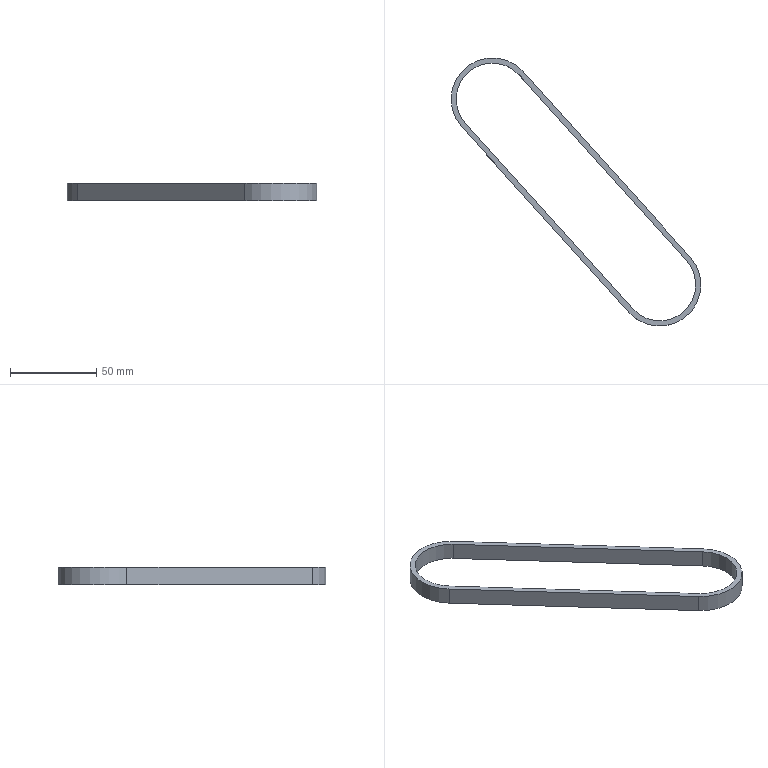Part | STEP file | 1 solid | 12 faces | box 145.075 x 155.71 x 10 mm | volume 12941 mm3 | plane 6 | cylinder 6 | commonest cylinder face diameters 42 x3 48 x3
STEP:
#1=CARTESIAN_POINT('',(0.,0.,0.));
#2=DIRECTION('',(0.,0.,1.));
#3=DIRECTION('',(1.,0.,0.));
#4=AXIS2_PLACEMENT_3D('',#1,#2,#3);
#5=CARTESIAN_POINT('',(15.599,14.059,-2.));
#6=VERTEX_POINT('',#5);
#7=CARTESIAN_POINT('',(-81.476,121.769,-2.));
#8=VERTEX_POINT('',#7);
#9=CARTESIAN_POINT('',(15.599,14.059,-2.));
#10=DIRECTION('',(-0.6695,0.7428,0.));
#11=VECTOR('',#10,1.);
#12=LINE('',#9,#11);
#13=CARTESIAN_POINT('',(15.599,14.059,-12.));
#14=DIRECTION('',(0.7428,0.6695,0.));
#15=DIRECTION('',(0.,0.,-1.));
#16=AXIS2_PLACEMENT_3D('',#13,#14,#15);
#17=PLANE('',#16);
#18=CARTESIAN_POINT('',(-10.,0.));
#19=DIRECTION('',(0.,1.));
#20=VECTOR('',#19,1.);
#21=LINE('',#18,#20);
#22=(GEOMETRIC_REPRESENTATION_CONTEXT(2)PARAMETRIC_REPRESENTATION_CONTEXT()REPRESENTATION_CONTEXT('',''));
#23=DEFINITIONAL_REPRESENTATION('',(#21),#22);
#24=PCURVE('',#17,#23);
#25=CARTESIAN_POINT('',(0.,0.,-2.));
#26=DIRECTION('',(0.,0.,1.));
#27=DIRECTION('',(1.,0.,0.));
#28=AXIS2_PLACEMENT_3D('',#25,#26,#27);
#29=PLANE('',#28);
#30=CARTESIAN_POINT('',(15.599,14.059));
#31=DIRECTION('',(-0.6695,0.7428));
#32=VECTOR('',#31,1.);
#33=LINE('',#30,#32);
#34=(GEOMETRIC_REPRESENTATION_CONTEXT(2)PARAMETRIC_REPRESENTATION_CONTEXT()REPRESENTATION_CONTEXT('',''));
#35=DEFINITIONAL_REPRESENTATION('',(#33),#34);
#36=PCURVE('',#29,#35);
#37=SURFACE_CURVE('',#12,(#24,#36),.PCURVE_S1.);
#38=EDGE_CURVE('',#6,#8,#37,.T.);
#39=ORIENTED_EDGE('',*,*,#38,.T.);
#40=CARTESIAN_POINT('',(-81.476,121.769,-12.));
#41=VERTEX_POINT('',#40);
#42=CARTESIAN_POINT('',(-81.476,121.769,-12.));
#43=DIRECTION('',(0.,0.,1.));
#44=VECTOR('',#43,1.);
#45=LINE('',#42,#44);
#46=CARTESIAN_POINT('',(0.,145.));
#47=DIRECTION('',(-1.,0.));
#48=VECTOR('',#47,1.);
#49=LINE('',#46,#48);
#50=(GEOMETRIC_REPRESENTATION_CONTEXT(2)PARAMETRIC_REPRESENTATION_CONTEXT()REPRESENTATION_CONTEXT('',''));
#51=DEFINITIONAL_REPRESENTATION('',(#49),#50);
#52=PCURVE('',#17,#51);
#53=CARTESIAN_POINT('',(-97.075,107.71,-12.));
#54=DIRECTION('',(0.,0.,1.));
#55=DIRECTION('',(1.,0.,0.));
#56=AXIS2_PLACEMENT_3D('',#53,#54,#55);
#57=CYLINDRICAL_SURFACE('',#56,21.);
#58=CARTESIAN_POINT('',(0.7335,0.));
#59=DIRECTION('',(0.,1.));
#60=VECTOR('',#59,1.);
#61=LINE('',#58,#60);
#62=(GEOMETRIC_REPRESENTATION_CONTEXT(2)PARAMETRIC_REPRESENTATION_CONTEXT()REPRESENTATION_CONTEXT('',''));
#63=DEFINITIONAL_REPRESENTATION('',(#61),#62);
#64=PCURVE('',#57,#63);
#65=SURFACE_CURVE('',#45,(#52,#64),.PCURVE_S1.);
#66=EDGE_CURVE('',#41,#8,#65,.T.);
#67=ORIENTED_EDGE('',*,*,#66,.F.);
#68=CARTESIAN_POINT('',(15.599,14.059,-12.));
#69=VERTEX_POINT('',#68);
#70=CARTESIAN_POINT('',(15.599,14.059,-12.));
#71=DIRECTION('',(-0.6695,0.7428,0.));
#72=VECTOR('',#71,1.);
#73=LINE('',#70,#72);
#74=CARTESIAN_POINT('',(0.,0.));
#75=DIRECTION('',(0.,1.));
#76=VECTOR('',#75,1.);
#77=LINE('',#74,#76);
#78=(GEOMETRIC_REPRESENTATION_CONTEXT(2)PARAMETRIC_REPRESENTATION_CONTEXT()REPRESENTATION_CONTEXT('',''));
#79=DEFINITIONAL_REPRESENTATION('',(#77),#78);
#80=PCURVE('',#17,#79);
#81=CARTESIAN_POINT('',(0.,0.,-12.));
#82=DIRECTION('',(0.,0.,1.));
#83=DIRECTION('',(1.,0.,0.));
#84=AXIS2_PLACEMENT_3D('',#81,#82,#83);
#85=PLANE('',#84);
#86=CARTESIAN_POINT('',(15.599,14.059));
#87=DIRECTION('',(-0.6695,0.7428));
#88=VECTOR('',#87,1.);
#89=LINE('',#86,#88);
#90=(GEOMETRIC_REPRESENTATION_CONTEXT(2)PARAMETRIC_REPRESENTATION_CONTEXT()REPRESENTATION_CONTEXT('',''));
#91=DEFINITIONAL_REPRESENTATION('',(#89),#90);
#92=PCURVE('',#85,#91);
#93=SURFACE_CURVE('',#73,(#80,#92),.PCURVE_S1.);
#94=EDGE_CURVE('',#69,#41,#93,.T.);
#95=ORIENTED_EDGE('',*,*,#94,.F.);
#96=CARTESIAN_POINT('',(15.599,14.059,-12.));
#97=DIRECTION('',(0.,0.,1.));
#98=VECTOR('',#97,1.);
#99=LINE('',#96,#98);
#100=CARTESIAN_POINT('',(0.,0.));
#101=DIRECTION('',(-1.,0.));
#102=VECTOR('',#101,1.);
#103=LINE('',#100,#102);
#104=(GEOMETRIC_REPRESENTATION_CONTEXT(2)PARAMETRIC_REPRESENTATION_CONTEXT()REPRESENTATION_CONTEXT('',''));
#105=DEFINITIONAL_REPRESENTATION('',(#103),#104);
#106=PCURVE('',#17,#105);
#107=CARTESIAN_POINT('',(0.,0.,-12.));
#108=DIRECTION('',(0.,0.,1.));
#109=DIRECTION('',(1.,0.,0.));
#110=AXIS2_PLACEMENT_3D('',#107,#108,#109);
#111=CYLINDRICAL_SURFACE('',#110,21.);
#112=CARTESIAN_POINT('',(0.7335,0.));
#113=DIRECTION('',(0.,1.));
#114=VECTOR('',#113,1.);
#115=LINE('',#112,#114);
#116=(GEOMETRIC_REPRESENTATION_CONTEXT(2)PARAMETRIC_REPRESENTATION_CONTEXT()REPRESENTATION_CONTEXT('',''));
#117=DEFINITIONAL_REPRESENTATION('',(#115),#116);
#118=PCURVE('',#111,#117);
#119=SURFACE_CURVE('',#99,(#106,#118),.PCURVE_S1.);
#120=EDGE_CURVE('',#69,#6,#119,.T.);
#121=ORIENTED_EDGE('',*,*,#120,.T.);
#122=EDGE_LOOP('',(#39,#67,#95,#121));
#123=FACE_BOUND('',#122,.T.);
#124=ADVANCED_FACE('',(#123),#17,.F.);
#125=ORIENTED_EDGE('',*,*,#66,.F.);
#126=CARTESIAN_POINT('',(-112.674,93.651,-12.));
#127=VERTEX_POINT('',#126);
#128=CARTESIAN_POINT('',(-97.075,107.71,-12.));
#129=DIRECTION('',(0.,0.,1.));
#130=DIRECTION('',(1.,0.,0.));
#131=AXIS2_PLACEMENT_3D('',#128,#129,#130);
#132=CIRCLE('',#131,21.);
#133=CARTESIAN_POINT('',(0.,0.));
#134=DIRECTION('',(1.,0.));
#135=VECTOR('',#134,1.);
#136=LINE('',#133,#135);
#137=(GEOMETRIC_REPRESENTATION_CONTEXT(2)PARAMETRIC_REPRESENTATION_CONTEXT()REPRESENTATION_CONTEXT('',''));
#138=DEFINITIONAL_REPRESENTATION('',(#136),#137);
#139=PCURVE('',#57,#138);
#140=CARTESIAN_POINT('',(-97.075,107.71));
#141=DIRECTION('',(1.,0.));
#142=AXIS2_PLACEMENT_2D('',#140,#141);
#143=CIRCLE('',#142,21.);
#144=(GEOMETRIC_REPRESENTATION_CONTEXT(2)PARAMETRIC_REPRESENTATION_CONTEXT()REPRESENTATION_CONTEXT('',''));
#145=DEFINITIONAL_REPRESENTATION('',(#143),#144);
#146=PCURVE('',#85,#145);
#147=SURFACE_CURVE('',#132,(#139,#146),.PCURVE_S1.);
#148=EDGE_CURVE('',#41,#127,#147,.T.);
#149=ORIENTED_EDGE('',*,*,#148,.T.);
#150=CARTESIAN_POINT('',(-112.674,93.651,-2.));
#151=VERTEX_POINT('',#150);
#152=CARTESIAN_POINT('',(-112.674,93.651,-12.));
#153=DIRECTION('',(0.,0.,1.));
#154=VECTOR('',#153,1.);
#155=LINE('',#152,#154);
#156=CARTESIAN_POINT('',(3.875,0.));
#157=DIRECTION('',(0.,1.));
#158=VECTOR('',#157,1.);
#159=LINE('',#156,#158);
#160=(GEOMETRIC_REPRESENTATION_CONTEXT(2)PARAMETRIC_REPRESENTATION_CONTEXT()REPRESENTATION_CONTEXT('',''));
#161=DEFINITIONAL_REPRESENTATION('',(#159),#160);
#162=PCURVE('',#57,#161);
#163=CARTESIAN_POINT('',(-15.599,-14.059,-12.));
#164=DIRECTION('',(-0.7428,-0.6695,0.));
#165=DIRECTION('',(-0.6695,0.7428,0.));
#166=AXIS2_PLACEMENT_3D('',#163,#164,#165);
#167=PLANE('',#166);
#168=CARTESIAN_POINT('',(145.,0.));
#169=DIRECTION('',(0.,-1.));
#170=VECTOR('',#169,1.);
#171=LINE('',#168,#170);
#172=(GEOMETRIC_REPRESENTATION_CONTEXT(2)PARAMETRIC_REPRESENTATION_CONTEXT()REPRESENTATION_CONTEXT('',''));
#173=DEFINITIONAL_REPRESENTATION('',(#171),#172);
#174=PCURVE('',#167,#173);
#175=SURFACE_CURVE('',#155,(#162,#174),.PCURVE_S1.);
#176=EDGE_CURVE('',#127,#151,#175,.T.);
#177=ORIENTED_EDGE('',*,*,#176,.T.);
#178=CARTESIAN_POINT('',(-97.075,107.71,-2.));
#179=DIRECTION('',(0.,0.,1.));
#180=DIRECTION('',(1.,0.,0.));
#181=AXIS2_PLACEMENT_3D('',#178,#179,#180);
#182=CIRCLE('',#181,21.);
#183=CARTESIAN_POINT('',(0.,10.));
#184=DIRECTION('',(1.,0.));
#185=VECTOR('',#184,1.);
#186=LINE('',#183,#185);
#187=(GEOMETRIC_REPRESENTATION_CONTEXT(2)PARAMETRIC_REPRESENTATION_CONTEXT()REPRESENTATION_CONTEXT('',''));
#188=DEFINITIONAL_REPRESENTATION('',(#186),#187);
#189=PCURVE('',#57,#188);
#190=CARTESIAN_POINT('',(-97.075,107.71));
#191=DIRECTION('',(1.,0.));
#192=AXIS2_PLACEMENT_2D('',#190,#191);
#193=CIRCLE('',#192,21.);
#194=(GEOMETRIC_REPRESENTATION_CONTEXT(2)PARAMETRIC_REPRESENTATION_CONTEXT()REPRESENTATION_CONTEXT('',''));
#195=DEFINITIONAL_REPRESENTATION('',(#193),#194);
#196=PCURVE('',#29,#195);
#197=SURFACE_CURVE('',#182,(#189,#196),.PCURVE_S1.);
#198=EDGE_CURVE('',#8,#151,#197,.T.);
#199=ORIENTED_EDGE('',*,*,#198,.F.);
#200=EDGE_LOOP('',(#125,#149,#177,#199));
#201=FACE_BOUND('',#200,.F.);
#202=ADVANCED_FACE('',(#201),#57,.F.);
#203=CARTESIAN_POINT('',(-15.599,-14.059,-2.));
#204=VERTEX_POINT('',#203);
#205=CARTESIAN_POINT('',(-15.599,-14.059,-2.));
#206=DIRECTION('',(0.6695,-0.7428,0.));
#207=VECTOR('',#206,1.);
#208=LINE('',#205,#207);
#209=CARTESIAN_POINT('',(0.,-10.));
#210=DIRECTION('',(-1.,0.));
#211=VECTOR('',#210,1.);
#212=LINE('',#209,#211);
#213=(GEOMETRIC_REPRESENTATION_CONTEXT(2)PARAMETRIC_REPRESENTATION_CONTEXT()REPRESENTATION_CONTEXT('',''));
#214=DEFINITIONAL_REPRESENTATION('',(#212),#213);
#215=PCURVE('',#167,#214);
#216=CARTESIAN_POINT('',(-15.599,-14.059));
#217=DIRECTION('',(0.6695,-0.7428));
#218=VECTOR('',#217,1.);
#219=LINE('',#216,#218);
#220=(GEOMETRIC_REPRESENTATION_CONTEXT(2)PARAMETRIC_REPRESENTATION_CONTEXT()REPRESENTATION_CONTEXT('',''));
#221=DEFINITIONAL_REPRESENTATION('',(#219),#220);
#222=PCURVE('',#29,#221);
#223=SURFACE_CURVE('',#208,(#215,#222),.PCURVE_S1.);
#224=EDGE_CURVE('',#151,#204,#223,.T.);
#225=ORIENTED_EDGE('',*,*,#224,.T.);
#226=CARTESIAN_POINT('',(-15.599,-14.059,-12.));
#227=VERTEX_POINT('',#226);
#228=CARTESIAN_POINT('',(-15.599,-14.059,-12.));
#229=DIRECTION('',(0.,0.,1.));
#230=VECTOR('',#229,1.);
#231=LINE('',#228,#230);
#232=CARTESIAN_POINT('',(0.,0.));
#233=DIRECTION('',(0.,-1.));
#234=VECTOR('',#233,1.);
#235=LINE('',#232,#234);
#236=(GEOMETRIC_REPRESENTATION_CONTEXT(2)PARAMETRIC_REPRESENTATION_CONTEXT()REPRESENTATION_CONTEXT('',''));
#237=DEFINITIONAL_REPRESENTATION('',(#235),#236);
#238=PCURVE('',#167,#237);
#239=CARTESIAN_POINT('',(0.,0.,-12.));
#240=DIRECTION('',(0.,0.,1.));
#241=DIRECTION('',(1.,0.,0.));
#242=AXIS2_PLACEMENT_3D('',#239,#240,#241);
#243=CYLINDRICAL_SURFACE('',#242,21.);
#244=CARTESIAN_POINT('',(3.875,0.));
#245=DIRECTION('',(0.,1.));
#246=VECTOR('',#245,1.);
#247=LINE('',#244,#246);
#248=(GEOMETRIC_REPRESENTATION_CONTEXT(2)PARAMETRIC_REPRESENTATION_CONTEXT()REPRESENTATION_CONTEXT('',''));
#249=DEFINITIONAL_REPRESENTATION('',(#247),#248);
#250=PCURVE('',#243,#249);
#251=SURFACE_CURVE('',#231,(#238,#250),.PCURVE_S1.);
#252=EDGE_CURVE('',#227,#204,#251,.T.);
#253=ORIENTED_EDGE('',*,*,#252,.F.);
#254=CARTESIAN_POINT('',(-15.599,-14.059,-12.));
#255=DIRECTION('',(0.6695,-0.7428,0.));
#256=VECTOR('',#255,1.);
#257=LINE('',#254,#256);
#258=CARTESIAN_POINT('',(0.,0.));
#259=DIRECTION('',(-1.,0.));
#260=VECTOR('',#259,1.);
#261=LINE('',#258,#260);
#262=(GEOMETRIC_REPRESENTATION_CONTEXT(2)PARAMETRIC_REPRESENTATION_CONTEXT()REPRESENTATION_CONTEXT('',''));
#263=DEFINITIONAL_REPRESENTATION('',(#261),#262);
#264=PCURVE('',#167,#263);
#265=CARTESIAN_POINT('',(-15.599,-14.059));
#266=DIRECTION('',(0.6695,-0.7428));
#267=VECTOR('',#266,1.);
#268=LINE('',#265,#267);
#269=(GEOMETRIC_REPRESENTATION_CONTEXT(2)PARAMETRIC_REPRESENTATION_CONTEXT()REPRESENTATION_CONTEXT('',''));
#270=DEFINITIONAL_REPRESENTATION('',(#268),#269);
#271=PCURVE('',#85,#270);
#272=SURFACE_CURVE('',#257,(#264,#271),.PCURVE_S1.);
#273=EDGE_CURVE('',#127,#227,#272,.T.);
#274=ORIENTED_EDGE('',*,*,#273,.F.);
#275=ORIENTED_EDGE('',*,*,#176,.T.);
#276=EDGE_LOOP('',(#225,#253,#274,#275));
#277=FACE_BOUND('',#276,.T.);
#278=ADVANCED_FACE('',(#277),#167,.F.);
#279=CARTESIAN_POINT('',(21.,0.,-2.));
#280=VERTEX_POINT('',#279);
#281=CARTESIAN_POINT('',(0.,0.,-2.));
#282=DIRECTION('',(0.,0.,1.));
#283=DIRECTION('',(1.,0.,0.));
#284=AXIS2_PLACEMENT_3D('',#281,#282,#283);
#285=CIRCLE('',#284,21.);
#286=CARTESIAN_POINT('',(0.,10.));
#287=DIRECTION('',(1.,0.));
#288=VECTOR('',#287,1.);
#289=LINE('',#286,#288);
#290=(GEOMETRIC_REPRESENTATION_CONTEXT(2)PARAMETRIC_REPRESENTATION_CONTEXT()REPRESENTATION_CONTEXT('',''));
#291=DEFINITIONAL_REPRESENTATION('',(#289),#290);
#292=PCURVE('',#243,#291);
#293=CARTESIAN_POINT('',(0.,0.));
#294=DIRECTION('',(1.,0.));
#295=AXIS2_PLACEMENT_2D('',#293,#294);
#296=CIRCLE('',#295,21.);
#297=(GEOMETRIC_REPRESENTATION_CONTEXT(2)PARAMETRIC_REPRESENTATION_CONTEXT()REPRESENTATION_CONTEXT('',''));
#298=DEFINITIONAL_REPRESENTATION('',(#296),#297);
#299=PCURVE('',#29,#298);
#300=SURFACE_CURVE('',#285,(#292,#299),.PCURVE_S1.);
#301=EDGE_CURVE('',#204,#280,#300,.T.);
#302=ORIENTED_EDGE('',*,*,#301,.F.);
#303=ORIENTED_EDGE('',*,*,#252,.F.);
#304=CARTESIAN_POINT('',(21.,0.,-12.));
#305=VERTEX_POINT('',#304);
#306=CARTESIAN_POINT('',(0.,0.,-12.));
#307=DIRECTION('',(0.,0.,1.));
#308=DIRECTION('',(1.,0.,0.));
#309=AXIS2_PLACEMENT_3D('',#306,#307,#308);
#310=CIRCLE('',#309,21.);
#311=CARTESIAN_POINT('',(0.,0.));
#312=DIRECTION('',(1.,0.));
#313=VECTOR('',#312,1.);
#314=LINE('',#311,#313);
#315=(GEOMETRIC_REPRESENTATION_CONTEXT(2)PARAMETRIC_REPRESENTATION_CONTEXT()REPRESENTATION_CONTEXT('',''));
#316=DEFINITIONAL_REPRESENTATION('',(#314),#315);
#317=PCURVE('',#243,#316);
#318=CARTESIAN_POINT('',(0.,0.));
#319=DIRECTION('',(1.,0.));
#320=AXIS2_PLACEMENT_2D('',#318,#319);
#321=CIRCLE('',#320,21.);
#322=(GEOMETRIC_REPRESENTATION_CONTEXT(2)PARAMETRIC_REPRESENTATION_CONTEXT()REPRESENTATION_CONTEXT('',''));
#323=DEFINITIONAL_REPRESENTATION('',(#321),#322);
#324=PCURVE('',#85,#323);
#325=SURFACE_CURVE('',#310,(#317,#324),.PCURVE_S1.);
#326=EDGE_CURVE('',#227,#305,#325,.T.);
#327=ORIENTED_EDGE('',*,*,#326,.T.);
#328=CARTESIAN_POINT('',(21.,0.,-12.));
#329=DIRECTION('',(0.,0.,1.));
#330=VECTOR('',#329,1.);
#331=LINE('',#328,#330);
#332=CARTESIAN_POINT('',(6.283,0.));
#333=DIRECTION('',(0.,1.));
#334=VECTOR('',#333,1.);
#335=LINE('',#332,#334);
#336=(GEOMETRIC_REPRESENTATION_CONTEXT(2)PARAMETRIC_REPRESENTATION_CONTEXT()REPRESENTATION_CONTEXT('',''));
#337=DEFINITIONAL_REPRESENTATION('',(#335),#336);
#338=PCURVE('',#243,#337);
#339=CARTESIAN_POINT('',(0.,0.));
#340=DIRECTION('',(0.,1.));
#341=VECTOR('',#340,1.);
#342=LINE('',#339,#341);
#343=(GEOMETRIC_REPRESENTATION_CONTEXT(2)PARAMETRIC_REPRESENTATION_CONTEXT()REPRESENTATION_CONTEXT('',''));
#344=DEFINITIONAL_REPRESENTATION('',(#342),#343);
#345=PCURVE('',#111,#344);
#346=SURFACE_CURVE('',#331,(#338,#345),.PCURVE_S1.);
#347=EDGE_CURVE('',#305,#280,#346,.T.);
#348=ORIENTED_EDGE('',*,*,#347,.T.);
#349=EDGE_LOOP('',(#302,#303,#327,#348));
#350=FACE_BOUND('',#349,.F.);
#351=ADVANCED_FACE('',(#350),#243,.F.);
#352=ORIENTED_EDGE('',*,*,#301,.F.);
#353=ORIENTED_EDGE('',*,*,#224,.F.);
#354=ORIENTED_EDGE('',*,*,#198,.F.);
#355=ORIENTED_EDGE('',*,*,#38,.F.);
#356=CARTESIAN_POINT('',(0.,0.,-2.));
#357=DIRECTION('',(0.,0.,1.));
#358=DIRECTION('',(1.,0.,0.));
#359=AXIS2_PLACEMENT_3D('',#356,#357,#358);
#360=CIRCLE('',#359,21.);
#361=CARTESIAN_POINT('',(0.,0.));
#362=DIRECTION('',(1.,0.));
#363=AXIS2_PLACEMENT_2D('',#361,#362);
#364=CIRCLE('',#363,21.);
#365=(GEOMETRIC_REPRESENTATION_CONTEXT(2)PARAMETRIC_REPRESENTATION_CONTEXT()REPRESENTATION_CONTEXT('',''));
#366=DEFINITIONAL_REPRESENTATION('',(#364),#365);
#367=PCURVE('',#29,#366);
#368=CARTESIAN_POINT('',(0.,10.));
#369=DIRECTION('',(1.,0.));
#370=VECTOR('',#369,1.);
#371=LINE('',#368,#370);
#372=(GEOMETRIC_REPRESENTATION_CONTEXT(2)PARAMETRIC_REPRESENTATION_CONTEXT()REPRESENTATION_CONTEXT('',''));
#373=DEFINITIONAL_REPRESENTATION('',(#371),#372);
#374=PCURVE('',#111,#373);
#375=SURFACE_CURVE('',#360,(#367,#374),.PCURVE_S1.);
#376=EDGE_CURVE('',#280,#6,#375,.T.);
#377=ORIENTED_EDGE('',*,*,#376,.F.);
#378=EDGE_LOOP('',(#352,#353,#354,#355,#377));
#379=FACE_BOUND('',#378,.T.);
#380=CARTESIAN_POINT('',(-17.828,-16.068,-2.));
#381=VERTEX_POINT('',#380);
#382=CARTESIAN_POINT('',(24.,0.,-2.));
#383=VERTEX_POINT('',#382);
#384=CARTESIAN_POINT('',(0.,0.,-2.));
#385=DIRECTION('',(0.,0.,1.));
#386=DIRECTION('',(1.,0.,0.));
#387=AXIS2_PLACEMENT_3D('',#384,#385,#386);
#388=CIRCLE('',#387,24.);
#389=CARTESIAN_POINT('',(0.,0.));
#390=DIRECTION('',(1.,0.));
#391=AXIS2_PLACEMENT_2D('',#389,#390);
#392=CIRCLE('',#391,24.);
#393=(GEOMETRIC_REPRESENTATION_CONTEXT(2)PARAMETRIC_REPRESENTATION_CONTEXT()REPRESENTATION_CONTEXT('',''));
#394=DEFINITIONAL_REPRESENTATION('',(#392),#393);
#395=PCURVE('',#29,#394);
#396=CARTESIAN_POINT('',(0.,0.,-12.));
#397=DIRECTION('',(0.,0.,1.));
#398=DIRECTION('',(1.,0.,0.));
#399=AXIS2_PLACEMENT_3D('',#396,#397,#398);
#400=CYLINDRICAL_SURFACE('',#399,24.);
#401=CARTESIAN_POINT('',(0.,10.));
#402=DIRECTION('',(1.,0.));
#403=VECTOR('',#402,1.);
#404=LINE('',#401,#403);
#405=(GEOMETRIC_REPRESENTATION_CONTEXT(2)PARAMETRIC_REPRESENTATION_CONTEXT()REPRESENTATION_CONTEXT('',''));
#406=DEFINITIONAL_REPRESENTATION('',(#404),#405);
#407=PCURVE('',#400,#406);
#408=SURFACE_CURVE('',#388,(#395,#407),.PCURVE_S1.);
#409=EDGE_CURVE('',#381,#383,#408,.T.);
#410=ORIENTED_EDGE('',*,*,#409,.T.);
#411=CARTESIAN_POINT('',(17.828,16.068,-2.));
#412=VERTEX_POINT('',#411);
#413=CARTESIAN_POINT('',(0.,0.,-2.));
#414=DIRECTION('',(0.,0.,1.));
#415=DIRECTION('',(1.,0.,0.));
#416=AXIS2_PLACEMENT_3D('',#413,#414,#415);
#417=CIRCLE('',#416,24.);
#418=CARTESIAN_POINT('',(0.,0.));
#419=DIRECTION('',(1.,0.));
#420=AXIS2_PLACEMENT_2D('',#418,#419);
#421=CIRCLE('',#420,24.);
#422=(GEOMETRIC_REPRESENTATION_CONTEXT(2)PARAMETRIC_REPRESENTATION_CONTEXT()REPRESENTATION_CONTEXT('',''));
#423=DEFINITIONAL_REPRESENTATION('',(#421),#422);
#424=PCURVE('',#29,#423);
#425=CARTESIAN_POINT('',(0.,0.,-12.));
#426=DIRECTION('',(0.,0.,1.));
#427=DIRECTION('',(1.,0.,0.));
#428=AXIS2_PLACEMENT_3D('',#425,#426,#427);
#429=CYLINDRICAL_SURFACE('',#428,24.);
#430=CARTESIAN_POINT('',(0.,10.));
#431=DIRECTION('',(1.,0.));
#432=VECTOR('',#431,1.);
#433=LINE('',#430,#432);
#434=(GEOMETRIC_REPRESENTATION_CONTEXT(2)PARAMETRIC_REPRESENTATION_CONTEXT()REPRESENTATION_CONTEXT('',''));
#435=DEFINITIONAL_REPRESENTATION('',(#433),#434);
#436=PCURVE('',#429,#435);
#437=SURFACE_CURVE('',#417,(#424,#436),.PCURVE_S1.);
#438=EDGE_CURVE('',#383,#412,#437,.T.);
#439=ORIENTED_EDGE('',*,*,#438,.T.);
#440=CARTESIAN_POINT('',(-79.247,123.778,-2.));
#441=VERTEX_POINT('',#440);
#442=CARTESIAN_POINT('',(17.828,16.068,-2.));
#443=DIRECTION('',(-0.6695,0.7428,0.));
#444=VECTOR('',#443,1.);
#445=LINE('',#442,#444);
#446=CARTESIAN_POINT('',(17.828,16.068));
#447=DIRECTION('',(-0.6695,0.7428));
#448=VECTOR('',#447,1.);
#449=LINE('',#446,#448);
#450=(GEOMETRIC_REPRESENTATION_CONTEXT(2)PARAMETRIC_REPRESENTATION_CONTEXT()REPRESENTATION_CONTEXT('',''));
#451=DEFINITIONAL_REPRESENTATION('',(#449),#450);
#452=PCURVE('',#29,#451);
#453=CARTESIAN_POINT('',(17.828,16.068,-12.));
#454=DIRECTION('',(0.7428,0.6695,0.));
#455=DIRECTION('',(0.,0.,-1.));
#456=AXIS2_PLACEMENT_3D('',#453,#454,#455);
#457=PLANE('',#456);
#458=CARTESIAN_POINT('',(-10.,0.));
#459=DIRECTION('',(0.,1.));
#460=VECTOR('',#459,1.);
#461=LINE('',#458,#460);
#462=(GEOMETRIC_REPRESENTATION_CONTEXT(2)PARAMETRIC_REPRESENTATION_CONTEXT()REPRESENTATION_CONTEXT('',''));
#463=DEFINITIONAL_REPRESENTATION('',(#461),#462);
#464=PCURVE('',#457,#463);
#465=SURFACE_CURVE('',#445,(#452,#464),.PCURVE_S1.);
#466=EDGE_CURVE('',#412,#441,#465,.T.);
#467=ORIENTED_EDGE('',*,*,#466,.T.);
#468=CARTESIAN_POINT('',(-114.903,91.642,-2.));
#469=VERTEX_POINT('',#468);
#470=CARTESIAN_POINT('',(-97.075,107.71,-2.));
#471=DIRECTION('',(0.,0.,1.));
#472=DIRECTION('',(1.,0.,0.));
#473=AXIS2_PLACEMENT_3D('',#470,#471,#472);
#474=CIRCLE('',#473,24.);
#475=CARTESIAN_POINT('',(-97.075,107.71));
#476=DIRECTION('',(1.,0.));
#477=AXIS2_PLACEMENT_2D('',#475,#476);
#478=CIRCLE('',#477,24.);
#479=(GEOMETRIC_REPRESENTATION_CONTEXT(2)PARAMETRIC_REPRESENTATION_CONTEXT()REPRESENTATION_CONTEXT('',''));
#480=DEFINITIONAL_REPRESENTATION('',(#478),#479);
#481=PCURVE('',#29,#480);
#482=CARTESIAN_POINT('',(-97.075,107.71,-12.));
#483=DIRECTION('',(0.,0.,1.));
#484=DIRECTION('',(1.,0.,0.));
#485=AXIS2_PLACEMENT_3D('',#482,#483,#484);
#486=CYLINDRICAL_SURFACE('',#485,24.);
#487=CARTESIAN_POINT('',(0.,10.));
#488=DIRECTION('',(1.,0.));
#489=VECTOR('',#488,1.);
#490=LINE('',#487,#489);
#491=(GEOMETRIC_REPRESENTATION_CONTEXT(2)PARAMETRIC_REPRESENTATION_CONTEXT()REPRESENTATION_CONTEXT('',''));
#492=DEFINITIONAL_REPRESENTATION('',(#490),#491);
#493=PCURVE('',#486,#492);
#494=SURFACE_CURVE('',#474,(#481,#493),.PCURVE_S1.);
#495=EDGE_CURVE('',#441,#469,#494,.T.);
#496=ORIENTED_EDGE('',*,*,#495,.T.);
#497=CARTESIAN_POINT('',(-17.828,-16.068,-2.));
#498=DIRECTION('',(0.6695,-0.7428,0.));
#499=VECTOR('',#498,1.);
#500=LINE('',#497,#499);
#501=CARTESIAN_POINT('',(-17.828,-16.068));
#502=DIRECTION('',(0.6695,-0.7428));
#503=VECTOR('',#502,1.);
#504=LINE('',#501,#503);
#505=(GEOMETRIC_REPRESENTATION_CONTEXT(2)PARAMETRIC_REPRESENTATION_CONTEXT()REPRESENTATION_CONTEXT('',''));
#506=DEFINITIONAL_REPRESENTATION('',(#504),#505);
#507=PCURVE('',#29,#506);
#508=CARTESIAN_POINT('',(-17.828,-16.068,-12.));
#509=DIRECTION('',(-0.7428,-0.6695,0.));
#510=DIRECTION('',(-0.6695,0.7428,0.));
#511=AXIS2_PLACEMENT_3D('',#508,#509,#510);
#512=PLANE('',#511);
#513=CARTESIAN_POINT('',(0.,-10.));
#514=DIRECTION('',(-1.,0.));
#515=VECTOR('',#514,1.);
#516=LINE('',#513,#515);
#517=(GEOMETRIC_REPRESENTATION_CONTEXT(2)PARAMETRIC_REPRESENTATION_CONTEXT()REPRESENTATION_CONTEXT('',''));
#518=DEFINITIONAL_REPRESENTATION('',(#516),#517);
#519=PCURVE('',#512,#518);
#520=SURFACE_CURVE('',#500,(#507,#519),.PCURVE_S1.);
#521=EDGE_CURVE('',#469,#381,#520,.T.);
#522=ORIENTED_EDGE('',*,*,#521,.T.);
#523=EDGE_LOOP('',(#410,#439,#467,#496,#522));
#524=FACE_BOUND('',#523,.T.);
#525=ADVANCED_FACE('',(#379,#524),#29,.T.);
#526=ORIENTED_EDGE('',*,*,#273,.T.);
#527=ORIENTED_EDGE('',*,*,#326,.T.);
#528=CARTESIAN_POINT('',(0.,0.,-12.));
#529=DIRECTION('',(0.,0.,1.));
#530=DIRECTION('',(1.,0.,0.));
#531=AXIS2_PLACEMENT_3D('',#528,#529,#530);
#532=CIRCLE('',#531,21.);
#533=CARTESIAN_POINT('',(0.,0.));
#534=DIRECTION('',(1.,0.));
#535=AXIS2_PLACEMENT_2D('',#533,#534);
#536=CIRCLE('',#535,21.);
#537=(GEOMETRIC_REPRESENTATION_CONTEXT(2)PARAMETRIC_REPRESENTATION_CONTEXT()REPRESENTATION_CONTEXT('',''));
#538=DEFINITIONAL_REPRESENTATION('',(#536),#537);
#539=PCURVE('',#85,#538);
#540=CARTESIAN_POINT('',(0.,0.));
#541=DIRECTION('',(1.,0.));
#542=VECTOR('',#541,1.);
#543=LINE('',#540,#542);
#544=(GEOMETRIC_REPRESENTATION_CONTEXT(2)PARAMETRIC_REPRESENTATION_CONTEXT()REPRESENTATION_CONTEXT('',''));
#545=DEFINITIONAL_REPRESENTATION('',(#543),#544);
#546=PCURVE('',#111,#545);
#547=SURFACE_CURVE('',#532,(#539,#546),.PCURVE_S1.);
#548=EDGE_CURVE('',#305,#69,#547,.T.);
#549=ORIENTED_EDGE('',*,*,#548,.T.);
#550=ORIENTED_EDGE('',*,*,#94,.T.);
#551=ORIENTED_EDGE('',*,*,#148,.T.);
#552=EDGE_LOOP('',(#526,#527,#549,#550,#551));
#553=FACE_BOUND('',#552,.T.);
#554=CARTESIAN_POINT('',(-17.828,-16.068,-12.));
#555=VERTEX_POINT('',#554);
#556=CARTESIAN_POINT('',(24.,0.,-12.));
#557=VERTEX_POINT('',#556);
#558=CARTESIAN_POINT('',(0.,0.,-12.));
#559=DIRECTION('',(0.,0.,1.));
#560=DIRECTION('',(1.,0.,0.));
#561=AXIS2_PLACEMENT_3D('',#558,#559,#560);
#562=CIRCLE('',#561,24.);
#563=CARTESIAN_POINT('',(0.,0.));
#564=DIRECTION('',(1.,0.));
#565=AXIS2_PLACEMENT_2D('',#563,#564);
#566=CIRCLE('',#565,24.);
#567=(GEOMETRIC_REPRESENTATION_CONTEXT(2)PARAMETRIC_REPRESENTATION_CONTEXT()REPRESENTATION_CONTEXT('',''));
#568=DEFINITIONAL_REPRESENTATION('',(#566),#567);
#569=PCURVE('',#85,#568);
#570=CARTESIAN_POINT('',(0.,0.));
#571=DIRECTION('',(1.,0.));
#572=VECTOR('',#571,1.);
#573=LINE('',#570,#572);
#574=(GEOMETRIC_REPRESENTATION_CONTEXT(2)PARAMETRIC_REPRESENTATION_CONTEXT()REPRESENTATION_CONTEXT('',''));
#575=DEFINITIONAL_REPRESENTATION('',(#573),#574);
#576=PCURVE('',#400,#575);
#577=SURFACE_CURVE('',#562,(#569,#576),.PCURVE_S1.);
#578=EDGE_CURVE('',#555,#557,#577,.T.);
#579=ORIENTED_EDGE('',*,*,#578,.F.);
#580=CARTESIAN_POINT('',(-114.903,91.642,-12.));
#581=VERTEX_POINT('',#580);
#582=CARTESIAN_POINT('',(-17.828,-16.068,-12.));
#583=DIRECTION('',(0.6695,-0.7428,0.));
#584=VECTOR('',#583,1.);
#585=LINE('',#582,#584);
#586=CARTESIAN_POINT('',(-17.828,-16.068));
#587=DIRECTION('',(0.6695,-0.7428));
#588=VECTOR('',#587,1.);
#589=LINE('',#586,#588);
#590=(GEOMETRIC_REPRESENTATION_CONTEXT(2)PARAMETRIC_REPRESENTATION_CONTEXT()REPRESENTATION_CONTEXT('',''));
#591=DEFINITIONAL_REPRESENTATION('',(#589),#590);
#592=PCURVE('',#85,#591);
#593=CARTESIAN_POINT('',(0.,0.));
#594=DIRECTION('',(-1.,0.));
#595=VECTOR('',#594,1.);
#596=LINE('',#593,#595);
#597=(GEOMETRIC_REPRESENTATION_CONTEXT(2)PARAMETRIC_REPRESENTATION_CONTEXT()REPRESENTATION_CONTEXT('',''));
#598=DEFINITIONAL_REPRESENTATION('',(#596),#597);
#599=PCURVE('',#512,#598);
#600=SURFACE_CURVE('',#585,(#592,#599),.PCURVE_S1.);
#601=EDGE_CURVE('',#581,#555,#600,.T.);
#602=ORIENTED_EDGE('',*,*,#601,.F.);
#603=CARTESIAN_POINT('',(-79.247,123.778,-12.));
#604=VERTEX_POINT('',#603);
#605=CARTESIAN_POINT('',(-97.075,107.71,-12.));
#606=DIRECTION('',(0.,0.,1.));
#607=DIRECTION('',(1.,0.,0.));
#608=AXIS2_PLACEMENT_3D('',#605,#606,#607);
#609=CIRCLE('',#608,24.);
#610=CARTESIAN_POINT('',(-97.075,107.71));
#611=DIRECTION('',(1.,0.));
#612=AXIS2_PLACEMENT_2D('',#610,#611);
#613=CIRCLE('',#612,24.);
#614=(GEOMETRIC_REPRESENTATION_CONTEXT(2)PARAMETRIC_REPRESENTATION_CONTEXT()REPRESENTATION_CONTEXT('',''));
#615=DEFINITIONAL_REPRESENTATION('',(#613),#614);
#616=PCURVE('',#85,#615);
#617=CARTESIAN_POINT('',(0.,0.));
#618=DIRECTION('',(1.,0.));
#619=VECTOR('',#618,1.);
#620=LINE('',#617,#619);
#621=(GEOMETRIC_REPRESENTATION_CONTEXT(2)PARAMETRIC_REPRESENTATION_CONTEXT()REPRESENTATION_CONTEXT('',''));
#622=DEFINITIONAL_REPRESENTATION('',(#620),#621);
#623=PCURVE('',#486,#622);
#624=SURFACE_CURVE('',#609,(#616,#623),.PCURVE_S1.);
#625=EDGE_CURVE('',#604,#581,#624,.T.);
#626=ORIENTED_EDGE('',*,*,#625,.F.);
#627=CARTESIAN_POINT('',(17.828,16.068,-12.));
#628=VERTEX_POINT('',#627);
#629=CARTESIAN_POINT('',(17.828,16.068,-12.));
#630=DIRECTION('',(-0.6695,0.7428,0.));
#631=VECTOR('',#630,1.);
#632=LINE('',#629,#631);
#633=CARTESIAN_POINT('',(17.828,16.068));
#634=DIRECTION('',(-0.6695,0.7428));
#635=VECTOR('',#634,1.);
#636=LINE('',#633,#635);
#637=(GEOMETRIC_REPRESENTATION_CONTEXT(2)PARAMETRIC_REPRESENTATION_CONTEXT()REPRESENTATION_CONTEXT('',''));
#638=DEFINITIONAL_REPRESENTATION('',(#636),#637);
#639=PCURVE('',#85,#638);
#640=CARTESIAN_POINT('',(0.,0.));
#641=DIRECTION('',(0.,1.));
#642=VECTOR('',#641,1.);
#643=LINE('',#640,#642);
#644=(GEOMETRIC_REPRESENTATION_CONTEXT(2)PARAMETRIC_REPRESENTATION_CONTEXT()REPRESENTATION_CONTEXT('',''));
#645=DEFINITIONAL_REPRESENTATION('',(#643),#644);
#646=PCURVE('',#457,#645);
#647=SURFACE_CURVE('',#632,(#639,#646),.PCURVE_S1.);
#648=EDGE_CURVE('',#628,#604,#647,.T.);
#649=ORIENTED_EDGE('',*,*,#648,.F.);
#650=CARTESIAN_POINT('',(0.,0.,-12.));
#651=DIRECTION('',(0.,0.,1.));
#652=DIRECTION('',(1.,0.,0.));
#653=AXIS2_PLACEMENT_3D('',#650,#651,#652);
#654=CIRCLE('',#653,24.);
#655=CARTESIAN_POINT('',(0.,0.));
#656=DIRECTION('',(1.,0.));
#657=AXIS2_PLACEMENT_2D('',#655,#656);
#658=CIRCLE('',#657,24.);
#659=(GEOMETRIC_REPRESENTATION_CONTEXT(2)PARAMETRIC_REPRESENTATION_CONTEXT()REPRESENTATION_CONTEXT('',''));
#660=DEFINITIONAL_REPRESENTATION('',(#658),#659);
#661=PCURVE('',#85,#660);
#662=CARTESIAN_POINT('',(0.,0.));
#663=DIRECTION('',(1.,0.));
#664=VECTOR('',#663,1.);
#665=LINE('',#662,#664);
#666=(GEOMETRIC_REPRESENTATION_CONTEXT(2)PARAMETRIC_REPRESENTATION_CONTEXT()REPRESENTATION_CONTEXT('',''));
#667=DEFINITIONAL_REPRESENTATION('',(#665),#666);
#668=PCURVE('',#429,#667);
#669=SURFACE_CURVE('',#654,(#661,#668),.PCURVE_S1.);
#670=EDGE_CURVE('',#557,#628,#669,.T.);
#671=ORIENTED_EDGE('',*,*,#670,.F.);
#672=EDGE_LOOP('',(#579,#602,#626,#649,#671));
#673=FACE_BOUND('',#672,.T.);
#674=ADVANCED_FACE('',(#553,#673),#85,.F.);
#675=ORIENTED_EDGE('',*,*,#466,.F.);
#676=CARTESIAN_POINT('',(17.828,16.068,-12.));
#677=DIRECTION('',(0.,0.,1.));
#678=VECTOR('',#677,1.);
#679=LINE('',#676,#678);
#680=CARTESIAN_POINT('',(0.,0.));
#681=DIRECTION('',(-1.,0.));
#682=VECTOR('',#681,1.);
#683=LINE('',#680,#682);
#684=(GEOMETRIC_REPRESENTATION_CONTEXT(2)PARAMETRIC_REPRESENTATION_CONTEXT()REPRESENTATION_CONTEXT('',''));
#685=DEFINITIONAL_REPRESENTATION('',(#683),#684);
#686=PCURVE('',#457,#685);
#687=CARTESIAN_POINT('',(0.7335,0.));
#688=DIRECTION('',(0.,1.));
#689=VECTOR('',#688,1.);
#690=LINE('',#687,#689);
#691=(GEOMETRIC_REPRESENTATION_CONTEXT(2)PARAMETRIC_REPRESENTATION_CONTEXT()REPRESENTATION_CONTEXT('',''));
#692=DEFINITIONAL_REPRESENTATION('',(#690),#691);
#693=PCURVE('',#429,#692);
#694=SURFACE_CURVE('',#679,(#686,#693),.PCURVE_S1.);
#695=EDGE_CURVE('',#628,#412,#694,.T.);
#696=ORIENTED_EDGE('',*,*,#695,.F.);
#697=ORIENTED_EDGE('',*,*,#648,.T.);
#698=CARTESIAN_POINT('',(-79.247,123.778,-12.));
#699=DIRECTION('',(0.,0.,1.));
#700=VECTOR('',#699,1.);
#701=LINE('',#698,#700);
#702=CARTESIAN_POINT('',(0.,145.));
#703=DIRECTION('',(-1.,0.));
#704=VECTOR('',#703,1.);
#705=LINE('',#702,#704);
#706=(GEOMETRIC_REPRESENTATION_CONTEXT(2)PARAMETRIC_REPRESENTATION_CONTEXT()REPRESENTATION_CONTEXT('',''));
#707=DEFINITIONAL_REPRESENTATION('',(#705),#706);
#708=PCURVE('',#457,#707);
#709=CARTESIAN_POINT('',(0.7335,0.));
#710=DIRECTION('',(0.,1.));
#711=VECTOR('',#710,1.);
#712=LINE('',#709,#711);
#713=(GEOMETRIC_REPRESENTATION_CONTEXT(2)PARAMETRIC_REPRESENTATION_CONTEXT()REPRESENTATION_CONTEXT('',''));
#714=DEFINITIONAL_REPRESENTATION('',(#712),#713);
#715=PCURVE('',#486,#714);
#716=SURFACE_CURVE('',#701,(#708,#715),.PCURVE_S1.);
#717=EDGE_CURVE('',#604,#441,#716,.T.);
#718=ORIENTED_EDGE('',*,*,#717,.T.);
#719=EDGE_LOOP('',(#675,#696,#697,#718));
#720=FACE_BOUND('',#719,.T.);
#721=ADVANCED_FACE('',(#720),#457,.T.);
#722=ORIENTED_EDGE('',*,*,#495,.F.);
#723=ORIENTED_EDGE('',*,*,#717,.F.);
#724=ORIENTED_EDGE('',*,*,#625,.T.);
#725=CARTESIAN_POINT('',(-114.903,91.642,-12.));
#726=DIRECTION('',(0.,0.,1.));
#727=VECTOR('',#726,1.);
#728=LINE('',#725,#727);
#729=CARTESIAN_POINT('',(3.875,0.));
#730=DIRECTION('',(0.,1.));
#731=VECTOR('',#730,1.);
#732=LINE('',#729,#731);
#733=(GEOMETRIC_REPRESENTATION_CONTEXT(2)PARAMETRIC_REPRESENTATION_CONTEXT()REPRESENTATION_CONTEXT('',''));
#734=DEFINITIONAL_REPRESENTATION('',(#732),#733);
#735=PCURVE('',#486,#734);
#736=CARTESIAN_POINT('',(145.,0.));
#737=DIRECTION('',(0.,-1.));
#738=VECTOR('',#737,1.);
#739=LINE('',#736,#738);
#740=(GEOMETRIC_REPRESENTATION_CONTEXT(2)PARAMETRIC_REPRESENTATION_CONTEXT()REPRESENTATION_CONTEXT('',''));
#741=DEFINITIONAL_REPRESENTATION('',(#739),#740);
#742=PCURVE('',#512,#741);
#743=SURFACE_CURVE('',#728,(#735,#742),.PCURVE_S1.);
#744=EDGE_CURVE('',#581,#469,#743,.T.);
#745=ORIENTED_EDGE('',*,*,#744,.T.);
#746=EDGE_LOOP('',(#722,#723,#724,#745));
#747=FACE_BOUND('',#746,.T.);
#748=ADVANCED_FACE('',(#747),#486,.T.);
#749=ORIENTED_EDGE('',*,*,#521,.F.);
#750=ORIENTED_EDGE('',*,*,#744,.F.);
#751=ORIENTED_EDGE('',*,*,#601,.T.);
#752=CARTESIAN_POINT('',(-17.828,-16.068,-12.));
#753=DIRECTION('',(0.,0.,1.));
#754=VECTOR('',#753,1.);
#755=LINE('',#752,#754);
#756=CARTESIAN_POINT('',(0.,0.));
#757=DIRECTION('',(0.,-1.));
#758=VECTOR('',#757,1.);
#759=LINE('',#756,#758);
#760=(GEOMETRIC_REPRESENTATION_CONTEXT(2)PARAMETRIC_REPRESENTATION_CONTEXT()REPRESENTATION_CONTEXT('',''));
#761=DEFINITIONAL_REPRESENTATION('',(#759),#760);
#762=PCURVE('',#512,#761);
#763=CARTESIAN_POINT('',(3.875,0.));
#764=DIRECTION('',(0.,1.));
#765=VECTOR('',#764,1.);
#766=LINE('',#763,#765);
#767=(GEOMETRIC_REPRESENTATION_CONTEXT(2)PARAMETRIC_REPRESENTATION_CONTEXT()REPRESENTATION_CONTEXT('',''));
#768=DEFINITIONAL_REPRESENTATION('',(#766),#767);
#769=PCURVE('',#400,#768);
#770=SURFACE_CURVE('',#755,(#762,#769),.PCURVE_S1.);
#771=EDGE_CURVE('',#555,#381,#770,.T.);
#772=ORIENTED_EDGE('',*,*,#771,.T.);
#773=EDGE_LOOP('',(#749,#750,#751,#772));
#774=FACE_BOUND('',#773,.T.);
#775=ADVANCED_FACE('',(#774),#512,.T.);
#776=CARTESIAN_POINT('',(24.,0.,-12.));
#777=DIRECTION('',(0.,0.,1.));
#778=VECTOR('',#777,1.);
#779=LINE('',#776,#778);
#780=CARTESIAN_POINT('',(0.,0.));
#781=DIRECTION('',(0.,1.));
#782=VECTOR('',#781,1.);
#783=LINE('',#780,#782);
#784=(GEOMETRIC_REPRESENTATION_CONTEXT(2)PARAMETRIC_REPRESENTATION_CONTEXT()REPRESENTATION_CONTEXT('',''));
#785=DEFINITIONAL_REPRESENTATION('',(#783),#784);
#786=PCURVE('',#429,#785);
#787=CARTESIAN_POINT('',(6.283,0.));
#788=DIRECTION('',(0.,1.));
#789=VECTOR('',#788,1.);
#790=LINE('',#787,#789);
#791=(GEOMETRIC_REPRESENTATION_CONTEXT(2)PARAMETRIC_REPRESENTATION_CONTEXT()REPRESENTATION_CONTEXT('',''));
#792=DEFINITIONAL_REPRESENTATION('',(#790),#791);
#793=PCURVE('',#400,#792);
#794=SURFACE_CURVE('',#779,(#786,#793),.PCURVE_S1.);
#795=EDGE_CURVE('',#557,#383,#794,.T.);
#796=ORIENTED_EDGE('',*,*,#795,.F.);
#797=ORIENTED_EDGE('',*,*,#670,.T.);
#798=ORIENTED_EDGE('',*,*,#695,.T.);
#799=ORIENTED_EDGE('',*,*,#438,.F.);
#800=EDGE_LOOP('',(#796,#797,#798,#799));
#801=FACE_BOUND('',#800,.T.);
#802=ADVANCED_FACE('',(#801),#429,.T.);
#803=ORIENTED_EDGE('',*,*,#578,.T.);
#804=ORIENTED_EDGE('',*,*,#795,.T.);
#805=ORIENTED_EDGE('',*,*,#409,.F.);
#806=ORIENTED_EDGE('',*,*,#771,.F.);
#807=EDGE_LOOP('',(#803,#804,#805,#806));
#808=FACE_BOUND('',#807,.T.);
#809=ADVANCED_FACE('',(#808),#400,.T.);
#810=ORIENTED_EDGE('',*,*,#120,.T.);
#811=ORIENTED_EDGE('',*,*,#376,.F.);
#812=ORIENTED_EDGE('',*,*,#347,.F.);
#813=ORIENTED_EDGE('',*,*,#548,.T.);
#814=EDGE_LOOP('',(#810,#811,#812,#813));
#815=FACE_BOUND('',#814,.F.);
#816=ADVANCED_FACE('',(#815),#111,.F.);
#817=CLOSED_SHELL('',(#124,#202,#278,#351,#525,#674,#721,#748,#775,#802,#809,#816));
#818=MANIFOLD_SOLID_BREP('',#817);
#819=(LENGTH_UNIT()NAMED_UNIT(*)SI_UNIT(.MILLI.,.METRE.));
#820=UNCERTAINTY_MEASURE_WITH_UNIT(LENGTH_MEASURE(0.0000001),#819,'','');
#821=(NAMED_UNIT(*)PLANE_ANGLE_UNIT()SI_UNIT($,.RADIAN.));
#822=(NAMED_UNIT(*)SI_UNIT($,.STERADIAN.)SOLID_ANGLE_UNIT());
#823=(GEOMETRIC_REPRESENTATION_CONTEXT(3)GLOBAL_UNCERTAINTY_ASSIGNED_CONTEXT((#820))GLOBAL_UNIT_ASSIGNED_CONTEXT((#819,#821,#822))REPRESENTATION_CONTEXT('',''));
#824=ADVANCED_BREP_SHAPE_REPRESENTATION('',(#4,#818),#823);